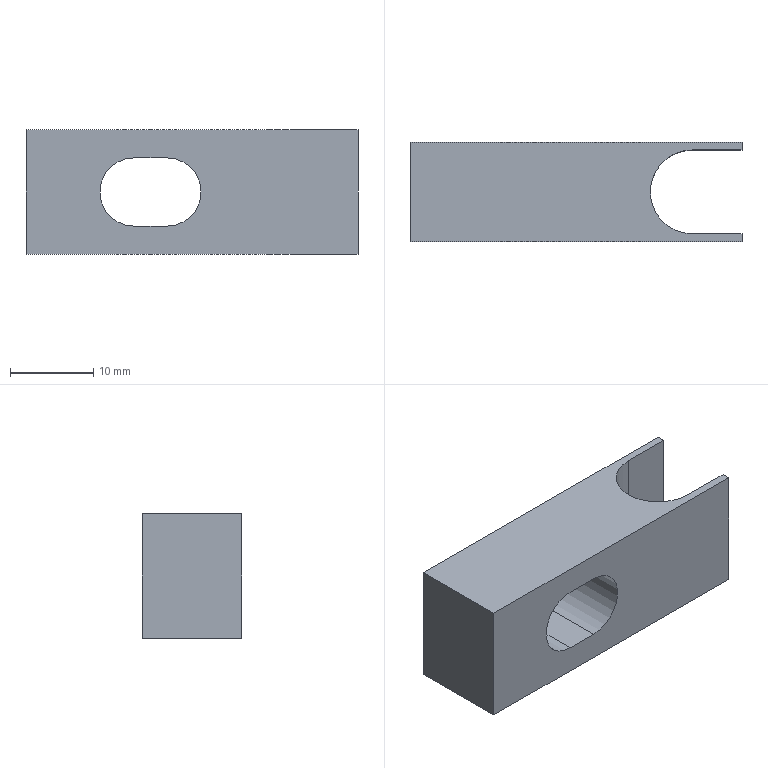Part | STEP file | Lead screw movable block QY-1-18 | 1 solid | 15 faces | box 40 x 12 x 15 mm | volume 4663 mm3 | plane 11 | cylinder 4 | commonest cylinder face diameters 8.2 x2 10.1 x2
STEP:
#1=CARTESIAN_POINT('',(0.,0.,0.));
#2=DIRECTION('',(0.,0.,1.));
#3=DIRECTION('',(1.,0.,0.));
#4=AXIS2_PLACEMENT_3D('',#1,#2,#3);
#5=CARTESIAN_POINT('',(9.9,2.027,15.));
#6=VERTEX_POINT('',#5);
#7=CARTESIAN_POINT('',(9.9,2.027,0.));
#8=VERTEX_POINT('',#7);
#9=CARTESIAN_POINT('',(9.9,2.027,15.));
#10=DIRECTION('',(0.,0.,-1.));
#11=VECTOR('',#10,1.);
#12=LINE('',#9,#11);
#13=CARTESIAN_POINT('',(9.9,-3.023,15.));
#14=DIRECTION('',(0.,0.,-1.));
#15=DIRECTION('',(-1.,0.,0.));
#16=AXIS2_PLACEMENT_3D('',#13,#14,#15);
#17=CYLINDRICAL_SURFACE('',#16,5.05);
#18=CARTESIAN_POINT('',(1.571,0.));
#19=DIRECTION('',(0.,1.));
#20=VECTOR('',#19,1.);
#21=LINE('',#18,#20);
#22=(GEOMETRIC_REPRESENTATION_CONTEXT(2)PARAMETRIC_REPRESENTATION_CONTEXT()REPRESENTATION_CONTEXT('',''));
#23=DEFINITIONAL_REPRESENTATION('',(#21),#22);
#24=PCURVE('',#17,#23);
#25=CARTESIAN_POINT('',(9.9,2.027,15.));
#26=DIRECTION('',(0.,1.,0.));
#27=DIRECTION('',(0.,0.,1.));
#28=AXIS2_PLACEMENT_3D('',#25,#26,#27);
#29=PLANE('',#28);
#30=CARTESIAN_POINT('',(0.,0.));
#31=DIRECTION('',(-1.,0.));
#32=VECTOR('',#31,1.);
#33=LINE('',#30,#32);
#34=(GEOMETRIC_REPRESENTATION_CONTEXT(2)PARAMETRIC_REPRESENTATION_CONTEXT()REPRESENTATION_CONTEXT('',''));
#35=DEFINITIONAL_REPRESENTATION('',(#33),#34);
#36=PCURVE('',#29,#35);
#37=SURFACE_CURVE('',#12,(#24,#36),.PCURVE_S1.);
#38=EDGE_CURVE('',#6,#8,#37,.T.);
#39=ORIENTED_EDGE('',*,*,#38,.T.);
#40=CARTESIAN_POINT('',(4.85,-3.023,0.));
#41=VERTEX_POINT('',#40);
#42=CARTESIAN_POINT('',(9.9,-3.023,0.));
#43=DIRECTION('',(0.,0.,-1.));
#44=DIRECTION('',(1.,0.,0.));
#45=AXIS2_PLACEMENT_3D('',#42,#43,#44);
#46=CIRCLE('',#45,5.05);
#47=CARTESIAN_POINT('',(-3.142,15.));
#48=DIRECTION('',(1.,0.));
#49=VECTOR('',#48,1.);
#50=LINE('',#47,#49);
#51=(GEOMETRIC_REPRESENTATION_CONTEXT(2)PARAMETRIC_REPRESENTATION_CONTEXT()REPRESENTATION_CONTEXT('',''));
#52=DEFINITIONAL_REPRESENTATION('',(#50),#51);
#53=PCURVE('',#17,#52);
#54=CARTESIAN_POINT('',(9.9,-3.023,0.));
#55=DIRECTION('',(0.,0.,1.));
#56=DIRECTION('',(1.,0.,0.));
#57=AXIS2_PLACEMENT_3D('',#54,#55,#56);
#58=PLANE('',#57);
#59=CARTESIAN_POINT('',(5.05,0.));
#60=CARTESIAN_POINT('',(5.05,-8.747));
#61=CARTESIAN_POINT('',(-2.525,-4.373));
#62=CARTESIAN_POINT('',(-10.1,0.));
#63=CARTESIAN_POINT('',(-2.525,4.373));
#64=CARTESIAN_POINT('',(5.05,8.747));
#65=CARTESIAN_POINT('',(5.05,0.));
#66=(BOUNDED_CURVE()B_SPLINE_CURVE(2,(#59,#60,#61,#62,#63,#64,#65),.UNSPECIFIED.,.T.,.F.)B_SPLINE_CURVE_WITH_KNOTS((1,2,2,2,2,1),(-2.094,0.,2.094,4.189,6.283,8.378),.UNSPECIFIED.)CURVE()GEOMETRIC_REPRESENTATION_ITEM()RATIONAL_B_SPLINE_CURVE((1.,0.5,1.,0.5,1.,0.5,1.))REPRESENTATION_ITEM(''));
#67=(GEOMETRIC_REPRESENTATION_CONTEXT(2)PARAMETRIC_REPRESENTATION_CONTEXT()REPRESENTATION_CONTEXT('',''));
#68=DEFINITIONAL_REPRESENTATION('',(#66),#67);
#69=PCURVE('',#58,#68);
#70=SURFACE_CURVE('',#46,(#53,#69),.PCURVE_S1.);
#71=EDGE_CURVE('',#41,#8,#70,.T.);
#72=ORIENTED_EDGE('',*,*,#71,.F.);
#73=CARTESIAN_POINT('',(4.85,-3.023,15.));
#74=VERTEX_POINT('',#73);
#75=CARTESIAN_POINT('',(4.85,-3.023,15.));
#76=DIRECTION('',(0.,0.,-1.));
#77=VECTOR('',#76,1.);
#78=LINE('',#75,#77);
#79=CARTESIAN_POINT('',(0.,0.));
#80=DIRECTION('',(0.,1.));
#81=VECTOR('',#80,1.);
#82=LINE('',#79,#81);
#83=(GEOMETRIC_REPRESENTATION_CONTEXT(2)PARAMETRIC_REPRESENTATION_CONTEXT()REPRESENTATION_CONTEXT('',''));
#84=DEFINITIONAL_REPRESENTATION('',(#82),#83);
#85=PCURVE('',#17,#84);
#86=CARTESIAN_POINT('',(9.9,-3.023,15.));
#87=DIRECTION('',(0.,0.,-1.));
#88=DIRECTION('',(-1.,0.,0.));
#89=AXIS2_PLACEMENT_3D('',#86,#87,#88);
#90=CYLINDRICAL_SURFACE('',#89,5.05);
#91=CARTESIAN_POINT('',(6.283,0.));
#92=DIRECTION('',(0.,1.));
#93=VECTOR('',#92,1.);
#94=LINE('',#91,#93);
#95=(GEOMETRIC_REPRESENTATION_CONTEXT(2)PARAMETRIC_REPRESENTATION_CONTEXT()REPRESENTATION_CONTEXT('',''));
#96=DEFINITIONAL_REPRESENTATION('',(#94),#95);
#97=PCURVE('',#90,#96);
#98=SURFACE_CURVE('',#78,(#85,#97),.PCURVE_S1.);
#99=EDGE_CURVE('',#74,#41,#98,.T.);
#100=ORIENTED_EDGE('',*,*,#99,.F.);
#101=CARTESIAN_POINT('',(9.9,-3.023,15.));
#102=DIRECTION('',(0.,0.,-1.));
#103=DIRECTION('',(1.,0.,0.));
#104=AXIS2_PLACEMENT_3D('',#101,#102,#103);
#105=CIRCLE('',#104,5.05);
#106=CARTESIAN_POINT('',(-3.142,0.));
#107=DIRECTION('',(1.,0.));
#108=VECTOR('',#107,1.);
#109=LINE('',#106,#108);
#110=(GEOMETRIC_REPRESENTATION_CONTEXT(2)PARAMETRIC_REPRESENTATION_CONTEXT()REPRESENTATION_CONTEXT('',''));
#111=DEFINITIONAL_REPRESENTATION('',(#109),#110);
#112=PCURVE('',#17,#111);
#113=CARTESIAN_POINT('',(9.9,-3.023,15.));
#114=DIRECTION('',(0.,0.,1.));
#115=DIRECTION('',(1.,0.,0.));
#116=AXIS2_PLACEMENT_3D('',#113,#114,#115);
#117=PLANE('',#116);
#118=CARTESIAN_POINT('',(5.05,0.));
#119=CARTESIAN_POINT('',(5.05,-8.747));
#120=CARTESIAN_POINT('',(-2.525,-4.373));
#121=CARTESIAN_POINT('',(-10.1,0.));
#122=CARTESIAN_POINT('',(-2.525,4.373));
#123=CARTESIAN_POINT('',(5.05,8.747));
#124=CARTESIAN_POINT('',(5.05,0.));
#125=(BOUNDED_CURVE()B_SPLINE_CURVE(2,(#118,#119,#120,#121,#122,#123,#124),.UNSPECIFIED.,.T.,.F.)B_SPLINE_CURVE_WITH_KNOTS((1,2,2,2,2,1),(-2.094,0.,2.094,4.189,6.283,8.378),.UNSPECIFIED.)CURVE()GEOMETRIC_REPRESENTATION_ITEM()RATIONAL_B_SPLINE_CURVE((1.,0.5,1.,0.5,1.,0.5,1.))REPRESENTATION_ITEM(''));
#126=(GEOMETRIC_REPRESENTATION_CONTEXT(2)PARAMETRIC_REPRESENTATION_CONTEXT()REPRESENTATION_CONTEXT('',''));
#127=DEFINITIONAL_REPRESENTATION('',(#125),#126);
#128=PCURVE('',#117,#127);
#129=SURFACE_CURVE('',#105,(#112,#128),.PCURVE_S1.);
#130=EDGE_CURVE('',#74,#6,#129,.T.);
#131=ORIENTED_EDGE('',*,*,#130,.T.);
#132=EDGE_LOOP('',(#39,#72,#100,#131));
#133=FACE_BOUND('',#132,.F.);
#134=ADVANCED_FACE('',(#133),#17,.F.);
#135=CARTESIAN_POINT('',(-24.1,2.977,0.));
#136=VERTEX_POINT('',#135);
#137=CARTESIAN_POINT('',(-24.1,-9.023,0.));
#138=VERTEX_POINT('',#137);
#139=CARTESIAN_POINT('',(-24.1,2.977,0.));
#140=DIRECTION('',(0.,-1.,0.));
#141=VECTOR('',#140,1.);
#142=LINE('',#139,#141);
#143=CARTESIAN_POINT('',(-24.1,2.977,15.));
#144=DIRECTION('',(1.,0.,0.));
#145=DIRECTION('',(0.,0.,-1.));
#146=AXIS2_PLACEMENT_3D('',#143,#144,#145);
#147=PLANE('',#146);
#148=CARTESIAN_POINT('',(15.,0.));
#149=DIRECTION('',(0.,-1.));
#150=VECTOR('',#149,1.);
#151=LINE('',#148,#150);
#152=(GEOMETRIC_REPRESENTATION_CONTEXT(2)PARAMETRIC_REPRESENTATION_CONTEXT()REPRESENTATION_CONTEXT('',''));
#153=DEFINITIONAL_REPRESENTATION('',(#151),#152);
#154=PCURVE('',#147,#153);
#155=CARTESIAN_POINT('',(-34.,6.));
#156=DIRECTION('',(0.,-1.));
#157=VECTOR('',#156,1.);
#158=LINE('',#155,#157);
#159=(GEOMETRIC_REPRESENTATION_CONTEXT(2)PARAMETRIC_REPRESENTATION_CONTEXT()REPRESENTATION_CONTEXT('',''));
#160=DEFINITIONAL_REPRESENTATION('',(#158),#159);
#161=PCURVE('',#58,#160);
#162=SURFACE_CURVE('',#142,(#154,#161),.PCURVE_S1.);
#163=EDGE_CURVE('',#136,#138,#162,.T.);
#164=ORIENTED_EDGE('',*,*,#163,.T.);
#165=CARTESIAN_POINT('',(-24.1,-9.023,15.));
#166=VERTEX_POINT('',#165);
#167=CARTESIAN_POINT('',(-24.1,-9.023,15.));
#168=DIRECTION('',(0.,0.,-1.));
#169=VECTOR('',#168,1.);
#170=LINE('',#167,#169);
#171=CARTESIAN_POINT('',(0.,-12.));
#172=DIRECTION('',(1.,0.));
#173=VECTOR('',#172,1.);
#174=LINE('',#171,#173);
#175=(GEOMETRIC_REPRESENTATION_CONTEXT(2)PARAMETRIC_REPRESENTATION_CONTEXT()REPRESENTATION_CONTEXT('',''));
#176=DEFINITIONAL_REPRESENTATION('',(#174),#175);
#177=PCURVE('',#147,#176);
#178=CARTESIAN_POINT('',(-24.1,-9.023,15.));
#179=DIRECTION('',(0.,1.,0.));
#180=DIRECTION('',(0.,0.,1.));
#181=AXIS2_PLACEMENT_3D('',#178,#179,#180);
#182=PLANE('',#181);
#183=CARTESIAN_POINT('',(0.,0.));
#184=DIRECTION('',(-1.,0.));
#185=VECTOR('',#184,1.);
#186=LINE('',#183,#185);
#187=(GEOMETRIC_REPRESENTATION_CONTEXT(2)PARAMETRIC_REPRESENTATION_CONTEXT()REPRESENTATION_CONTEXT('',''));
#188=DEFINITIONAL_REPRESENTATION('',(#186),#187);
#189=PCURVE('',#182,#188);
#190=SURFACE_CURVE('',#170,(#177,#189),.PCURVE_S1.);
#191=EDGE_CURVE('',#166,#138,#190,.T.);
#192=ORIENTED_EDGE('',*,*,#191,.F.);
#193=CARTESIAN_POINT('',(-24.1,2.977,15.));
#194=VERTEX_POINT('',#193);
#195=CARTESIAN_POINT('',(-24.1,2.977,15.));
#196=DIRECTION('',(0.,-1.,0.));
#197=VECTOR('',#196,1.);
#198=LINE('',#195,#197);
#199=CARTESIAN_POINT('',(0.,0.));
#200=DIRECTION('',(0.,-1.));
#201=VECTOR('',#200,1.);
#202=LINE('',#199,#201);
#203=(GEOMETRIC_REPRESENTATION_CONTEXT(2)PARAMETRIC_REPRESENTATION_CONTEXT()REPRESENTATION_CONTEXT('',''));
#204=DEFINITIONAL_REPRESENTATION('',(#202),#203);
#205=PCURVE('',#147,#204);
#206=CARTESIAN_POINT('',(-34.,6.));
#207=DIRECTION('',(0.,-1.));
#208=VECTOR('',#207,1.);
#209=LINE('',#206,#208);
#210=(GEOMETRIC_REPRESENTATION_CONTEXT(2)PARAMETRIC_REPRESENTATION_CONTEXT()REPRESENTATION_CONTEXT('',''));
#211=DEFINITIONAL_REPRESENTATION('',(#209),#210);
#212=PCURVE('',#117,#211);
#213=SURFACE_CURVE('',#198,(#205,#212),.PCURVE_S1.);
#214=EDGE_CURVE('',#194,#166,#213,.T.);
#215=ORIENTED_EDGE('',*,*,#214,.F.);
#216=CARTESIAN_POINT('',(-24.1,2.977,15.));
#217=DIRECTION('',(0.,0.,-1.));
#218=VECTOR('',#217,1.);
#219=LINE('',#216,#218);
#220=CARTESIAN_POINT('',(0.,0.));
#221=DIRECTION('',(1.,0.));
#222=VECTOR('',#221,1.);
#223=LINE('',#220,#222);
#224=(GEOMETRIC_REPRESENTATION_CONTEXT(2)PARAMETRIC_REPRESENTATION_CONTEXT()REPRESENTATION_CONTEXT('',''));
#225=DEFINITIONAL_REPRESENTATION('',(#223),#224);
#226=PCURVE('',#147,#225);
#227=CARTESIAN_POINT('',(-24.1,2.977,15.));
#228=DIRECTION('',(0.,-1.,0.));
#229=DIRECTION('',(1.,0.,0.));
#230=AXIS2_PLACEMENT_3D('',#227,#228,#229);
#231=PLANE('',#230);
#232=CARTESIAN_POINT('',(0.,0.));
#233=DIRECTION('',(0.,-1.));
#234=VECTOR('',#233,1.);
#235=LINE('',#232,#234);
#236=(GEOMETRIC_REPRESENTATION_CONTEXT(2)PARAMETRIC_REPRESENTATION_CONTEXT()REPRESENTATION_CONTEXT('',''));
#237=DEFINITIONAL_REPRESENTATION('',(#235),#236);
#238=PCURVE('',#231,#237);
#239=SURFACE_CURVE('',#219,(#226,#238),.PCURVE_S1.);
#240=EDGE_CURVE('',#194,#136,#239,.T.);
#241=ORIENTED_EDGE('',*,*,#240,.T.);
#242=EDGE_LOOP('',(#164,#192,#215,#241));
#243=FACE_BOUND('',#242,.T.);
#244=ADVANCED_FACE('',(#243),#147,.F.);
#245=CARTESIAN_POINT('',(-7.1,-9.023,11.6));
#246=VERTEX_POINT('',#245);
#247=CARTESIAN_POINT('',(-11.1,-9.023,11.6));
#248=VERTEX_POINT('',#247);
#249=CARTESIAN_POINT('',(-7.1,-9.023,11.6));
#250=DIRECTION('',(-1.,0.,0.));
#251=VECTOR('',#250,1.);
#252=LINE('',#249,#251);
#253=CARTESIAN_POINT('',(-3.4,17.));
#254=DIRECTION('',(0.,-1.));
#255=VECTOR('',#254,1.);
#256=LINE('',#253,#255);
#257=(GEOMETRIC_REPRESENTATION_CONTEXT(2)PARAMETRIC_REPRESENTATION_CONTEXT()REPRESENTATION_CONTEXT('',''));
#258=DEFINITIONAL_REPRESENTATION('',(#256),#257);
#259=PCURVE('',#182,#258);
#260=CARTESIAN_POINT('',(-7.1,5.977,11.6));
#261=DIRECTION('',(0.,0.,1.));
#262=DIRECTION('',(1.,0.,0.));
#263=AXIS2_PLACEMENT_3D('',#260,#261,#262);
#264=PLANE('',#263);
#265=CARTESIAN_POINT('',(0.,-15.));
#266=DIRECTION('',(-1.,0.));
#267=VECTOR('',#266,1.);
#268=LINE('',#265,#267);
#269=(GEOMETRIC_REPRESENTATION_CONTEXT(2)PARAMETRIC_REPRESENTATION_CONTEXT()REPRESENTATION_CONTEXT('',''));
#270=DEFINITIONAL_REPRESENTATION('',(#268),#269);
#271=PCURVE('',#264,#270);
#272=SURFACE_CURVE('',#252,(#259,#271),.PCURVE_S1.);
#273=EDGE_CURVE('',#246,#248,#272,.T.);
#274=ORIENTED_EDGE('',*,*,#273,.F.);
#275=CARTESIAN_POINT('',(-7.1,-9.023,3.4));
#276=VERTEX_POINT('',#275);
#277=CARTESIAN_POINT('',(-7.1,-9.023,7.5));
#278=DIRECTION('',(0.,-1.,0.));
#279=DIRECTION('',(0.,0.,-1.));
#280=AXIS2_PLACEMENT_3D('',#277,#278,#279);
#281=CIRCLE('',#280,4.1);
#282=CARTESIAN_POINT('',(-11.6,17.));
#283=CARTESIAN_POINT('',(-11.6,24.101));
#284=CARTESIAN_POINT('',(-5.45,20.551));
#285=CARTESIAN_POINT('',(0.7,17.));
#286=CARTESIAN_POINT('',(-5.45,13.449));
#287=CARTESIAN_POINT('',(-11.6,9.899));
#288=CARTESIAN_POINT('',(-11.6,17.));
#289=(BOUNDED_CURVE()B_SPLINE_CURVE(2,(#282,#283,#284,#285,#286,#287,#288),.UNSPECIFIED.,.T.,.F.)B_SPLINE_CURVE_WITH_KNOTS((1,2,2,2,2,1),(-2.094,0.,2.094,4.189,6.283,8.378),.UNSPECIFIED.)CURVE()GEOMETRIC_REPRESENTATION_ITEM()RATIONAL_B_SPLINE_CURVE((1.,0.5,1.,0.5,1.,0.5,1.))REPRESENTATION_ITEM(''));
#290=(GEOMETRIC_REPRESENTATION_CONTEXT(2)PARAMETRIC_REPRESENTATION_CONTEXT()REPRESENTATION_CONTEXT('',''));
#291=DEFINITIONAL_REPRESENTATION('',(#289),#290);
#292=PCURVE('',#182,#291);
#293=CARTESIAN_POINT('',(-7.1,5.977,7.5));
#294=DIRECTION('',(0.,-1.,0.));
#295=DIRECTION('',(0.,0.,-1.));
#296=AXIS2_PLACEMENT_3D('',#293,#294,#295);
#297=CYLINDRICAL_SURFACE('',#296,4.1);
#298=CARTESIAN_POINT('',(0.,15.));
#299=DIRECTION('',(1.,0.));
#300=VECTOR('',#299,1.);
#301=LINE('',#298,#300);
#302=(GEOMETRIC_REPRESENTATION_CONTEXT(2)PARAMETRIC_REPRESENTATION_CONTEXT()REPRESENTATION_CONTEXT('',''));
#303=DEFINITIONAL_REPRESENTATION('',(#301),#302);
#304=PCURVE('',#297,#303);
#305=SURFACE_CURVE('',#281,(#292,#304),.PCURVE_S1.);
#306=EDGE_CURVE('',#276,#246,#305,.T.);
#307=ORIENTED_EDGE('',*,*,#306,.F.);
#308=CARTESIAN_POINT('',(-11.1,-9.023,3.4));
#309=VERTEX_POINT('',#308);
#310=CARTESIAN_POINT('',(-7.1,-9.023,3.4));
#311=DIRECTION('',(1.,0.,0.));
#312=VECTOR('',#311,1.);
#313=LINE('',#310,#312);
#314=CARTESIAN_POINT('',(-11.6,17.));
#315=DIRECTION('',(0.,1.));
#316=VECTOR('',#315,1.);
#317=LINE('',#314,#316);
#318=(GEOMETRIC_REPRESENTATION_CONTEXT(2)PARAMETRIC_REPRESENTATION_CONTEXT()REPRESENTATION_CONTEXT('',''));
#319=DEFINITIONAL_REPRESENTATION('',(#317),#318);
#320=PCURVE('',#182,#319);
#321=CARTESIAN_POINT('',(-7.1,5.977,3.4));
#322=DIRECTION('',(0.,0.,-1.));
#323=DIRECTION('',(-1.,0.,0.));
#324=AXIS2_PLACEMENT_3D('',#321,#322,#323);
#325=PLANE('',#324);
#326=CARTESIAN_POINT('',(0.,-15.));
#327=DIRECTION('',(-1.,0.));
#328=VECTOR('',#327,1.);
#329=LINE('',#326,#328);
#330=(GEOMETRIC_REPRESENTATION_CONTEXT(2)PARAMETRIC_REPRESENTATION_CONTEXT()REPRESENTATION_CONTEXT('',''));
#331=DEFINITIONAL_REPRESENTATION('',(#329),#330);
#332=PCURVE('',#325,#331);
#333=SURFACE_CURVE('',#313,(#320,#332),.PCURVE_S1.);
#334=EDGE_CURVE('',#309,#276,#333,.T.);
#335=ORIENTED_EDGE('',*,*,#334,.F.);
#336=CARTESIAN_POINT('',(-11.1,-9.023,7.5));
#337=DIRECTION('',(0.,-1.,0.));
#338=DIRECTION('',(0.,0.,-1.));
#339=AXIS2_PLACEMENT_3D('',#336,#337,#338);
#340=CIRCLE('',#339,4.1);
#341=CARTESIAN_POINT('',(-11.6,13.));
#342=CARTESIAN_POINT('',(-11.6,20.101));
#343=CARTESIAN_POINT('',(-5.45,16.551));
#344=CARTESIAN_POINT('',(0.7,13.));
#345=CARTESIAN_POINT('',(-5.45,9.449));
#346=CARTESIAN_POINT('',(-11.6,5.899));
#347=CARTESIAN_POINT('',(-11.6,13.));
#348=(BOUNDED_CURVE()B_SPLINE_CURVE(2,(#341,#342,#343,#344,#345,#346,#347),.UNSPECIFIED.,.T.,.F.)B_SPLINE_CURVE_WITH_KNOTS((1,2,2,2,2,1),(-2.094,0.,2.094,4.189,6.283,8.378),.UNSPECIFIED.)CURVE()GEOMETRIC_REPRESENTATION_ITEM()RATIONAL_B_SPLINE_CURVE((1.,0.5,1.,0.5,1.,0.5,1.))REPRESENTATION_ITEM(''));
#349=(GEOMETRIC_REPRESENTATION_CONTEXT(2)PARAMETRIC_REPRESENTATION_CONTEXT()REPRESENTATION_CONTEXT('',''));
#350=DEFINITIONAL_REPRESENTATION('',(#348),#349);
#351=PCURVE('',#182,#350);
#352=CARTESIAN_POINT('',(-11.1,5.977,7.5));
#353=DIRECTION('',(0.,-1.,0.));
#354=DIRECTION('',(0.,0.,-1.));
#355=AXIS2_PLACEMENT_3D('',#352,#353,#354);
#356=CYLINDRICAL_SURFACE('',#355,4.1);
#357=CARTESIAN_POINT('',(0.,15.));
#358=DIRECTION('',(1.,0.));
#359=VECTOR('',#358,1.);
#360=LINE('',#357,#359);
#361=(GEOMETRIC_REPRESENTATION_CONTEXT(2)PARAMETRIC_REPRESENTATION_CONTEXT()REPRESENTATION_CONTEXT('',''));
#362=DEFINITIONAL_REPRESENTATION('',(#360),#361);
#363=PCURVE('',#356,#362);
#364=SURFACE_CURVE('',#340,(#351,#363),.PCURVE_S1.);
#365=EDGE_CURVE('',#248,#309,#364,.T.);
#366=ORIENTED_EDGE('',*,*,#365,.F.);
#367=EDGE_LOOP('',(#274,#307,#335,#366));
#368=FACE_BOUND('',#367,.T.);
#369=CARTESIAN_POINT('',(15.9,-9.023,0.));
#370=VERTEX_POINT('',#369);
#371=CARTESIAN_POINT('',(-24.1,-9.023,0.));
#372=DIRECTION('',(1.,0.,0.));
#373=VECTOR('',#372,1.);
#374=LINE('',#371,#373);
#375=CARTESIAN_POINT('',(-15.,0.));
#376=DIRECTION('',(0.,1.));
#377=VECTOR('',#376,1.);
#378=LINE('',#375,#377);
#379=(GEOMETRIC_REPRESENTATION_CONTEXT(2)PARAMETRIC_REPRESENTATION_CONTEXT()REPRESENTATION_CONTEXT('',''));
#380=DEFINITIONAL_REPRESENTATION('',(#378),#379);
#381=PCURVE('',#182,#380);
#382=CARTESIAN_POINT('',(-34.,-6.));
#383=DIRECTION('',(1.,0.));
#384=VECTOR('',#383,1.);
#385=LINE('',#382,#384);
#386=(GEOMETRIC_REPRESENTATION_CONTEXT(2)PARAMETRIC_REPRESENTATION_CONTEXT()REPRESENTATION_CONTEXT('',''));
#387=DEFINITIONAL_REPRESENTATION('',(#385),#386);
#388=PCURVE('',#58,#387);
#389=SURFACE_CURVE('',#374,(#381,#388),.PCURVE_S1.);
#390=EDGE_CURVE('',#138,#370,#389,.T.);
#391=ORIENTED_EDGE('',*,*,#390,.T.);
#392=CARTESIAN_POINT('',(15.9,-9.023,15.));
#393=VERTEX_POINT('',#392);
#394=CARTESIAN_POINT('',(15.9,-9.023,15.));
#395=DIRECTION('',(0.,0.,-1.));
#396=VECTOR('',#395,1.);
#397=LINE('',#394,#396);
#398=CARTESIAN_POINT('',(0.,40.));
#399=DIRECTION('',(-1.,0.));
#400=VECTOR('',#399,1.);
#401=LINE('',#398,#400);
#402=(GEOMETRIC_REPRESENTATION_CONTEXT(2)PARAMETRIC_REPRESENTATION_CONTEXT()REPRESENTATION_CONTEXT('',''));
#403=DEFINITIONAL_REPRESENTATION('',(#401),#402);
#404=PCURVE('',#182,#403);
#405=CARTESIAN_POINT('',(15.9,-8.073,15.));
#406=DIRECTION('',(-1.,0.,0.));
#407=DIRECTION('',(0.,0.,1.));
#408=AXIS2_PLACEMENT_3D('',#405,#406,#407);
#409=PLANE('',#408);
#410=CARTESIAN_POINT('',(0.,-0.95));
#411=DIRECTION('',(-1.,0.));
#412=VECTOR('',#411,1.);
#413=LINE('',#410,#412);
#414=(GEOMETRIC_REPRESENTATION_CONTEXT(2)PARAMETRIC_REPRESENTATION_CONTEXT()REPRESENTATION_CONTEXT('',''));
#415=DEFINITIONAL_REPRESENTATION('',(#413),#414);
#416=PCURVE('',#409,#415);
#417=SURFACE_CURVE('',#397,(#404,#416),.PCURVE_S1.);
#418=EDGE_CURVE('',#393,#370,#417,.T.);
#419=ORIENTED_EDGE('',*,*,#418,.F.);
#420=CARTESIAN_POINT('',(-24.1,-9.023,15.));
#421=DIRECTION('',(1.,0.,0.));
#422=VECTOR('',#421,1.);
#423=LINE('',#420,#422);
#424=CARTESIAN_POINT('',(0.,0.));
#425=DIRECTION('',(0.,1.));
#426=VECTOR('',#425,1.);
#427=LINE('',#424,#426);
#428=(GEOMETRIC_REPRESENTATION_CONTEXT(2)PARAMETRIC_REPRESENTATION_CONTEXT()REPRESENTATION_CONTEXT('',''));
#429=DEFINITIONAL_REPRESENTATION('',(#427),#428);
#430=PCURVE('',#182,#429);
#431=CARTESIAN_POINT('',(-34.,-6.));
#432=DIRECTION('',(1.,0.));
#433=VECTOR('',#432,1.);
#434=LINE('',#431,#433);
#435=(GEOMETRIC_REPRESENTATION_CONTEXT(2)PARAMETRIC_REPRESENTATION_CONTEXT()REPRESENTATION_CONTEXT('',''));
#436=DEFINITIONAL_REPRESENTATION('',(#434),#435);
#437=PCURVE('',#117,#436);
#438=SURFACE_CURVE('',#423,(#430,#437),.PCURVE_S1.);
#439=EDGE_CURVE('',#166,#393,#438,.T.);
#440=ORIENTED_EDGE('',*,*,#439,.F.);
#441=ORIENTED_EDGE('',*,*,#191,.T.);
#442=EDGE_LOOP('',(#391,#419,#440,#441));
#443=FACE_BOUND('',#442,.T.);
#444=ADVANCED_FACE('',(#368,#443),#182,.F.);
#445=CARTESIAN_POINT('',(15.9,-8.073,0.));
#446=VERTEX_POINT('',#445);
#447=CARTESIAN_POINT('',(15.9,-8.073,0.));
#448=DIRECTION('',(0.,1.,0.));
#449=VECTOR('',#448,1.);
#450=LINE('',#447,#449);
#451=CARTESIAN_POINT('',(-15.,0.));
#452=DIRECTION('',(0.,1.));
#453=VECTOR('',#452,1.);
#454=LINE('',#451,#453);
#455=(GEOMETRIC_REPRESENTATION_CONTEXT(2)PARAMETRIC_REPRESENTATION_CONTEXT()REPRESENTATION_CONTEXT('',''));
#456=DEFINITIONAL_REPRESENTATION('',(#454),#455);
#457=PCURVE('',#409,#456);
#458=CARTESIAN_POINT('',(6.,-5.05));
#459=DIRECTION('',(0.,1.));
#460=VECTOR('',#459,1.);
#461=LINE('',#458,#460);
#462=(GEOMETRIC_REPRESENTATION_CONTEXT(2)PARAMETRIC_REPRESENTATION_CONTEXT()REPRESENTATION_CONTEXT('',''));
#463=DEFINITIONAL_REPRESENTATION('',(#461),#462);
#464=PCURVE('',#58,#463);
#465=SURFACE_CURVE('',#450,(#457,#464),.PCURVE_S1.);
#466=EDGE_CURVE('',#370,#446,#465,.T.);
#467=ORIENTED_EDGE('',*,*,#466,.T.);
#468=CARTESIAN_POINT('',(15.9,-8.073,15.));
#469=VERTEX_POINT('',#468);
#470=CARTESIAN_POINT('',(15.9,-8.073,15.));
#471=DIRECTION('',(0.,0.,-1.));
#472=VECTOR('',#471,1.);
#473=LINE('',#470,#472);
#474=CARTESIAN_POINT('',(0.,0.));
#475=DIRECTION('',(-1.,0.));
#476=VECTOR('',#475,1.);
#477=LINE('',#474,#476);
#478=(GEOMETRIC_REPRESENTATION_CONTEXT(2)PARAMETRIC_REPRESENTATION_CONTEXT()REPRESENTATION_CONTEXT('',''));
#479=DEFINITIONAL_REPRESENTATION('',(#477),#478);
#480=PCURVE('',#409,#479);
#481=CARTESIAN_POINT('',(9.9,-8.073,15.));
#482=DIRECTION('',(0.,-1.,0.));
#483=DIRECTION('',(0.,0.,-1.));
#484=AXIS2_PLACEMENT_3D('',#481,#482,#483);
#485=PLANE('',#484);
#486=CARTESIAN_POINT('',(0.,6.));
#487=DIRECTION('',(1.,0.));
#488=VECTOR('',#487,1.);
#489=LINE('',#486,#488);
#490=(GEOMETRIC_REPRESENTATION_CONTEXT(2)PARAMETRIC_REPRESENTATION_CONTEXT()REPRESENTATION_CONTEXT('',''));
#491=DEFINITIONAL_REPRESENTATION('',(#489),#490);
#492=PCURVE('',#485,#491);
#493=SURFACE_CURVE('',#473,(#480,#492),.PCURVE_S1.);
#494=EDGE_CURVE('',#469,#446,#493,.T.);
#495=ORIENTED_EDGE('',*,*,#494,.F.);
#496=CARTESIAN_POINT('',(15.9,-8.073,15.));
#497=DIRECTION('',(0.,1.,0.));
#498=VECTOR('',#497,1.);
#499=LINE('',#496,#498);
#500=CARTESIAN_POINT('',(0.,0.));
#501=DIRECTION('',(0.,1.));
#502=VECTOR('',#501,1.);
#503=LINE('',#500,#502);
#504=(GEOMETRIC_REPRESENTATION_CONTEXT(2)PARAMETRIC_REPRESENTATION_CONTEXT()REPRESENTATION_CONTEXT('',''));
#505=DEFINITIONAL_REPRESENTATION('',(#503),#504);
#506=PCURVE('',#409,#505);
#507=CARTESIAN_POINT('',(6.,-5.05));
#508=DIRECTION('',(0.,1.));
#509=VECTOR('',#508,1.);
#510=LINE('',#507,#509);
#511=(GEOMETRIC_REPRESENTATION_CONTEXT(2)PARAMETRIC_REPRESENTATION_CONTEXT()REPRESENTATION_CONTEXT('',''));
#512=DEFINITIONAL_REPRESENTATION('',(#510),#511);
#513=PCURVE('',#117,#512);
#514=SURFACE_CURVE('',#499,(#506,#513),.PCURVE_S1.);
#515=EDGE_CURVE('',#393,#469,#514,.T.);
#516=ORIENTED_EDGE('',*,*,#515,.F.);
#517=ORIENTED_EDGE('',*,*,#418,.T.);
#518=EDGE_LOOP('',(#467,#495,#516,#517));
#519=FACE_BOUND('',#518,.T.);
#520=ADVANCED_FACE('',(#519),#409,.F.);
#521=CARTESIAN_POINT('',(9.9,-8.073,0.));
#522=VERTEX_POINT('',#521);
#523=CARTESIAN_POINT('',(9.9,-8.073,0.));
#524=DIRECTION('',(-1.,0.,0.));
#525=VECTOR('',#524,1.);
#526=LINE('',#523,#525);
#527=CARTESIAN_POINT('',(15.,0.));
#528=DIRECTION('',(0.,-1.));
#529=VECTOR('',#528,1.);
#530=LINE('',#527,#529);
#531=(GEOMETRIC_REPRESENTATION_CONTEXT(2)PARAMETRIC_REPRESENTATION_CONTEXT()REPRESENTATION_CONTEXT('',''));
#532=DEFINITIONAL_REPRESENTATION('',(#530),#531);
#533=PCURVE('',#485,#532);
#534=CARTESIAN_POINT('',(0.,-5.05));
#535=DIRECTION('',(-1.,0.));
#536=VECTOR('',#535,1.);
#537=LINE('',#534,#536);
#538=(GEOMETRIC_REPRESENTATION_CONTEXT(2)PARAMETRIC_REPRESENTATION_CONTEXT()REPRESENTATION_CONTEXT('',''));
#539=DEFINITIONAL_REPRESENTATION('',(#537),#538);
#540=PCURVE('',#58,#539);
#541=SURFACE_CURVE('',#526,(#533,#540),.PCURVE_S1.);
#542=EDGE_CURVE('',#446,#522,#541,.T.);
#543=ORIENTED_EDGE('',*,*,#542,.T.);
#544=CARTESIAN_POINT('',(9.9,-8.073,15.));
#545=VERTEX_POINT('',#544);
#546=CARTESIAN_POINT('',(9.9,-8.073,15.));
#547=DIRECTION('',(0.,0.,-1.));
#548=VECTOR('',#547,1.);
#549=LINE('',#546,#548);
#550=CARTESIAN_POINT('',(0.,0.));
#551=DIRECTION('',(1.,0.));
#552=VECTOR('',#551,1.);
#553=LINE('',#550,#552);
#554=(GEOMETRIC_REPRESENTATION_CONTEXT(2)PARAMETRIC_REPRESENTATION_CONTEXT()REPRESENTATION_CONTEXT('',''));
#555=DEFINITIONAL_REPRESENTATION('',(#553),#554);
#556=PCURVE('',#485,#555);
#557=CARTESIAN_POINT('',(4.712,0.));
#558=DIRECTION('',(0.,1.));
#559=VECTOR('',#558,1.);
#560=LINE('',#557,#559);
#561=(GEOMETRIC_REPRESENTATION_CONTEXT(2)PARAMETRIC_REPRESENTATION_CONTEXT()REPRESENTATION_CONTEXT('',''));
#562=DEFINITIONAL_REPRESENTATION('',(#560),#561);
#563=PCURVE('',#90,#562);
#564=SURFACE_CURVE('',#549,(#556,#563),.PCURVE_S1.);
#565=EDGE_CURVE('',#545,#522,#564,.T.);
#566=ORIENTED_EDGE('',*,*,#565,.F.);
#567=CARTESIAN_POINT('',(9.9,-8.073,15.));
#568=DIRECTION('',(-1.,0.,0.));
#569=VECTOR('',#568,1.);
#570=LINE('',#567,#569);
#571=CARTESIAN_POINT('',(0.,0.));
#572=DIRECTION('',(0.,-1.));
#573=VECTOR('',#572,1.);
#574=LINE('',#571,#573);
#575=(GEOMETRIC_REPRESENTATION_CONTEXT(2)PARAMETRIC_REPRESENTATION_CONTEXT()REPRESENTATION_CONTEXT('',''));
#576=DEFINITIONAL_REPRESENTATION('',(#574),#575);
#577=PCURVE('',#485,#576);
#578=CARTESIAN_POINT('',(0.,-5.05));
#579=DIRECTION('',(-1.,0.));
#580=VECTOR('',#579,1.);
#581=LINE('',#578,#580);
#582=(GEOMETRIC_REPRESENTATION_CONTEXT(2)PARAMETRIC_REPRESENTATION_CONTEXT()REPRESENTATION_CONTEXT('',''));
#583=DEFINITIONAL_REPRESENTATION('',(#581),#582);
#584=PCURVE('',#117,#583);
#585=SURFACE_CURVE('',#570,(#577,#584),.PCURVE_S1.);
#586=EDGE_CURVE('',#469,#545,#585,.T.);
#587=ORIENTED_EDGE('',*,*,#586,.F.);
#588=ORIENTED_EDGE('',*,*,#494,.T.);
#589=EDGE_LOOP('',(#543,#566,#587,#588));
#590=FACE_BOUND('',#589,.T.);
#591=ADVANCED_FACE('',(#590),#485,.F.);
#592=CARTESIAN_POINT('',(9.9,-3.023,0.));
#593=DIRECTION('',(0.,0.,-1.));
#594=DIRECTION('',(1.,0.,0.));
#595=AXIS2_PLACEMENT_3D('',#592,#593,#594);
#596=CIRCLE('',#595,5.05);
#597=CARTESIAN_POINT('',(3.142,15.));
#598=DIRECTION('',(1.,0.));
#599=VECTOR('',#598,1.);
#600=LINE('',#597,#599);
#601=(GEOMETRIC_REPRESENTATION_CONTEXT(2)PARAMETRIC_REPRESENTATION_CONTEXT()REPRESENTATION_CONTEXT('',''));
#602=DEFINITIONAL_REPRESENTATION('',(#600),#601);
#603=PCURVE('',#90,#602);
#604=CARTESIAN_POINT('',(5.05,0.));
#605=CARTESIAN_POINT('',(5.05,-8.747));
#606=CARTESIAN_POINT('',(-2.525,-4.373));
#607=CARTESIAN_POINT('',(-10.1,0.));
#608=CARTESIAN_POINT('',(-2.525,4.373));
#609=CARTESIAN_POINT('',(5.05,8.747));
#610=CARTESIAN_POINT('',(5.05,0.));
#611=(BOUNDED_CURVE()B_SPLINE_CURVE(2,(#604,#605,#606,#607,#608,#609,#610),.UNSPECIFIED.,.T.,.F.)B_SPLINE_CURVE_WITH_KNOTS((1,2,2,2,2,1),(-2.094,0.,2.094,4.189,6.283,8.378),.UNSPECIFIED.)CURVE()GEOMETRIC_REPRESENTATION_ITEM()RATIONAL_B_SPLINE_CURVE((1.,0.5,1.,0.5,1.,0.5,1.))REPRESENTATION_ITEM(''));
#612=(GEOMETRIC_REPRESENTATION_CONTEXT(2)PARAMETRIC_REPRESENTATION_CONTEXT()REPRESENTATION_CONTEXT('',''));
#613=DEFINITIONAL_REPRESENTATION('',(#611),#612);
#614=PCURVE('',#58,#613);
#615=SURFACE_CURVE('',#596,(#603,#614),.PCURVE_S1.);
#616=EDGE_CURVE('',#522,#41,#615,.T.);
#617=ORIENTED_EDGE('',*,*,#616,.F.);
#618=ORIENTED_EDGE('',*,*,#565,.F.);
#619=CARTESIAN_POINT('',(9.9,-3.023,15.));
#620=DIRECTION('',(0.,0.,-1.));
#621=DIRECTION('',(1.,0.,0.));
#622=AXIS2_PLACEMENT_3D('',#619,#620,#621);
#623=CIRCLE('',#622,5.05);
#624=CARTESIAN_POINT('',(3.142,0.));
#625=DIRECTION('',(1.,0.));
#626=VECTOR('',#625,1.);
#627=LINE('',#624,#626);
#628=(GEOMETRIC_REPRESENTATION_CONTEXT(2)PARAMETRIC_REPRESENTATION_CONTEXT()REPRESENTATION_CONTEXT('',''));
#629=DEFINITIONAL_REPRESENTATION('',(#627),#628);
#630=PCURVE('',#90,#629);
#631=CARTESIAN_POINT('',(5.05,0.));
#632=CARTESIAN_POINT('',(5.05,-8.747));
#633=CARTESIAN_POINT('',(-2.525,-4.373));
#634=CARTESIAN_POINT('',(-10.1,0.));
#635=CARTESIAN_POINT('',(-2.525,4.373));
#636=CARTESIAN_POINT('',(5.05,8.747));
#637=CARTESIAN_POINT('',(5.05,0.));
#638=(BOUNDED_CURVE()B_SPLINE_CURVE(2,(#631,#632,#633,#634,#635,#636,#637),.UNSPECIFIED.,.T.,.F.)B_SPLINE_CURVE_WITH_KNOTS((1,2,2,2,2,1),(-2.094,0.,2.094,4.189,6.283,8.378),.UNSPECIFIED.)CURVE()GEOMETRIC_REPRESENTATION_ITEM()RATIONAL_B_SPLINE_CURVE((1.,0.5,1.,0.5,1.,0.5,1.))REPRESENTATION_ITEM(''));
#639=(GEOMETRIC_REPRESENTATION_CONTEXT(2)PARAMETRIC_REPRESENTATION_CONTEXT()REPRESENTATION_CONTEXT('',''));
#640=DEFINITIONAL_REPRESENTATION('',(#638),#639);
#641=PCURVE('',#117,#640);
#642=SURFACE_CURVE('',#623,(#630,#641),.PCURVE_S1.);
#643=EDGE_CURVE('',#545,#74,#642,.T.);
#644=ORIENTED_EDGE('',*,*,#643,.T.);
#645=ORIENTED_EDGE('',*,*,#99,.T.);
#646=EDGE_LOOP('',(#617,#618,#644,#645));
#647=FACE_BOUND('',#646,.F.);
#648=ADVANCED_FACE('',(#647),#90,.F.);
#649=CARTESIAN_POINT('',(15.9,2.027,0.));
#650=VERTEX_POINT('',#649);
#651=CARTESIAN_POINT('',(9.9,2.027,0.));
#652=DIRECTION('',(1.,0.,0.));
#653=VECTOR('',#652,1.);
#654=LINE('',#651,#653);
#655=CARTESIAN_POINT('',(-15.,0.));
#656=DIRECTION('',(0.,1.));
#657=VECTOR('',#656,1.);
#658=LINE('',#655,#657);
#659=(GEOMETRIC_REPRESENTATION_CONTEXT(2)PARAMETRIC_REPRESENTATION_CONTEXT()REPRESENTATION_CONTEXT('',''));
#660=DEFINITIONAL_REPRESENTATION('',(#658),#659);
#661=PCURVE('',#29,#660);
#662=CARTESIAN_POINT('',(0.,5.05));
#663=DIRECTION('',(1.,0.));
#664=VECTOR('',#663,1.);
#665=LINE('',#662,#664);
#666=(GEOMETRIC_REPRESENTATION_CONTEXT(2)PARAMETRIC_REPRESENTATION_CONTEXT()REPRESENTATION_CONTEXT('',''));
#667=DEFINITIONAL_REPRESENTATION('',(#665),#666);
#668=PCURVE('',#58,#667);
#669=SURFACE_CURVE('',#654,(#661,#668),.PCURVE_S1.);
#670=EDGE_CURVE('',#8,#650,#669,.T.);
#671=ORIENTED_EDGE('',*,*,#670,.T.);
#672=CARTESIAN_POINT('',(15.9,2.027,15.));
#673=VERTEX_POINT('',#672);
#674=CARTESIAN_POINT('',(15.9,2.027,15.));
#675=DIRECTION('',(0.,0.,-1.));
#676=VECTOR('',#675,1.);
#677=LINE('',#674,#676);
#678=CARTESIAN_POINT('',(0.,6.));
#679=DIRECTION('',(-1.,0.));
#680=VECTOR('',#679,1.);
#681=LINE('',#678,#680);
#682=(GEOMETRIC_REPRESENTATION_CONTEXT(2)PARAMETRIC_REPRESENTATION_CONTEXT()REPRESENTATION_CONTEXT('',''));
#683=DEFINITIONAL_REPRESENTATION('',(#681),#682);
#684=PCURVE('',#29,#683);
#685=CARTESIAN_POINT('',(15.9,2.977,15.));
#686=DIRECTION('',(-1.,0.,0.));
#687=DIRECTION('',(0.,0.,1.));
#688=AXIS2_PLACEMENT_3D('',#685,#686,#687);
#689=PLANE('',#688);
#690=CARTESIAN_POINT('',(0.,-0.95));
#691=DIRECTION('',(-1.,0.));
#692=VECTOR('',#691,1.);
#693=LINE('',#690,#692);
#694=(GEOMETRIC_REPRESENTATION_CONTEXT(2)PARAMETRIC_REPRESENTATION_CONTEXT()REPRESENTATION_CONTEXT('',''));
#695=DEFINITIONAL_REPRESENTATION('',(#693),#694);
#696=PCURVE('',#689,#695);
#697=SURFACE_CURVE('',#677,(#684,#696),.PCURVE_S1.);
#698=EDGE_CURVE('',#673,#650,#697,.T.);
#699=ORIENTED_EDGE('',*,*,#698,.F.);
#700=CARTESIAN_POINT('',(9.9,2.027,15.));
#701=DIRECTION('',(1.,0.,0.));
#702=VECTOR('',#701,1.);
#703=LINE('',#700,#702);
#704=CARTESIAN_POINT('',(0.,0.));
#705=DIRECTION('',(0.,1.));
#706=VECTOR('',#705,1.);
#707=LINE('',#704,#706);
#708=(GEOMETRIC_REPRESENTATION_CONTEXT(2)PARAMETRIC_REPRESENTATION_CONTEXT()REPRESENTATION_CONTEXT('',''));
#709=DEFINITIONAL_REPRESENTATION('',(#707),#708);
#710=PCURVE('',#29,#709);
#711=CARTESIAN_POINT('',(0.,5.05));
#712=DIRECTION('',(1.,0.));
#713=VECTOR('',#712,1.);
#714=LINE('',#711,#713);
#715=(GEOMETRIC_REPRESENTATION_CONTEXT(2)PARAMETRIC_REPRESENTATION_CONTEXT()REPRESENTATION_CONTEXT('',''));
#716=DEFINITIONAL_REPRESENTATION('',(#714),#715);
#717=PCURVE('',#117,#716);
#718=SURFACE_CURVE('',#703,(#710,#717),.PCURVE_S1.);
#719=EDGE_CURVE('',#6,#673,#718,.T.);
#720=ORIENTED_EDGE('',*,*,#719,.F.);
#721=ORIENTED_EDGE('',*,*,#38,.T.);
#722=EDGE_LOOP('',(#671,#699,#720,#721));
#723=FACE_BOUND('',#722,.T.);
#724=ADVANCED_FACE('',(#723),#29,.F.);
#725=CARTESIAN_POINT('',(15.9,2.977,0.));
#726=VERTEX_POINT('',#725);
#727=CARTESIAN_POINT('',(15.9,2.977,0.));
#728=DIRECTION('',(0.,1.,0.));
#729=VECTOR('',#728,1.);
#730=LINE('',#727,#729);
#731=CARTESIAN_POINT('',(-15.,0.));
#732=DIRECTION('',(0.,1.));
#733=VECTOR('',#732,1.);
#734=LINE('',#731,#733);
#735=(GEOMETRIC_REPRESENTATION_CONTEXT(2)PARAMETRIC_REPRESENTATION_CONTEXT()REPRESENTATION_CONTEXT('',''));
#736=DEFINITIONAL_REPRESENTATION('',(#734),#735);
#737=PCURVE('',#689,#736);
#738=CARTESIAN_POINT('',(6.,6.));
#739=DIRECTION('',(0.,1.));
#740=VECTOR('',#739,1.);
#741=LINE('',#738,#740);
#742=(GEOMETRIC_REPRESENTATION_CONTEXT(2)PARAMETRIC_REPRESENTATION_CONTEXT()REPRESENTATION_CONTEXT('',''));
#743=DEFINITIONAL_REPRESENTATION('',(#741),#742);
#744=PCURVE('',#58,#743);
#745=SURFACE_CURVE('',#730,(#737,#744),.PCURVE_S1.);
#746=EDGE_CURVE('',#650,#726,#745,.T.);
#747=ORIENTED_EDGE('',*,*,#746,.T.);
#748=CARTESIAN_POINT('',(15.9,2.977,15.));
#749=VERTEX_POINT('',#748);
#750=CARTESIAN_POINT('',(15.9,2.977,15.));
#751=DIRECTION('',(0.,0.,-1.));
#752=VECTOR('',#751,1.);
#753=LINE('',#750,#752);
#754=CARTESIAN_POINT('',(0.,0.));
#755=DIRECTION('',(-1.,0.));
#756=VECTOR('',#755,1.);
#757=LINE('',#754,#756);
#758=(GEOMETRIC_REPRESENTATION_CONTEXT(2)PARAMETRIC_REPRESENTATION_CONTEXT()REPRESENTATION_CONTEXT('',''));
#759=DEFINITIONAL_REPRESENTATION('',(#757),#758);
#760=PCURVE('',#689,#759);
#761=CARTESIAN_POINT('',(40.,0.));
#762=DIRECTION('',(0.,-1.));
#763=VECTOR('',#762,1.);
#764=LINE('',#761,#763);
#765=(GEOMETRIC_REPRESENTATION_CONTEXT(2)PARAMETRIC_REPRESENTATION_CONTEXT()REPRESENTATION_CONTEXT('',''));
#766=DEFINITIONAL_REPRESENTATION('',(#764),#765);
#767=PCURVE('',#231,#766);
#768=SURFACE_CURVE('',#753,(#760,#767),.PCURVE_S1.);
#769=EDGE_CURVE('',#749,#726,#768,.T.);
#770=ORIENTED_EDGE('',*,*,#769,.F.);
#771=CARTESIAN_POINT('',(15.9,2.977,15.));
#772=DIRECTION('',(0.,1.,0.));
#773=VECTOR('',#772,1.);
#774=LINE('',#771,#773);
#775=CARTESIAN_POINT('',(0.,0.));
#776=DIRECTION('',(0.,1.));
#777=VECTOR('',#776,1.);
#778=LINE('',#775,#777);
#779=(GEOMETRIC_REPRESENTATION_CONTEXT(2)PARAMETRIC_REPRESENTATION_CONTEXT()REPRESENTATION_CONTEXT('',''));
#780=DEFINITIONAL_REPRESENTATION('',(#778),#779);
#781=PCURVE('',#689,#780);
#782=CARTESIAN_POINT('',(6.,6.));
#783=DIRECTION('',(0.,1.));
#784=VECTOR('',#783,1.);
#785=LINE('',#782,#784);
#786=(GEOMETRIC_REPRESENTATION_CONTEXT(2)PARAMETRIC_REPRESENTATION_CONTEXT()REPRESENTATION_CONTEXT('',''));
#787=DEFINITIONAL_REPRESENTATION('',(#785),#786);
#788=PCURVE('',#117,#787);
#789=SURFACE_CURVE('',#774,(#781,#788),.PCURVE_S1.);
#790=EDGE_CURVE('',#673,#749,#789,.T.);
#791=ORIENTED_EDGE('',*,*,#790,.F.);
#792=ORIENTED_EDGE('',*,*,#698,.T.);
#793=EDGE_LOOP('',(#747,#770,#791,#792));
#794=FACE_BOUND('',#793,.T.);
#795=ADVANCED_FACE('',(#794),#689,.F.);
#796=CARTESIAN_POINT('',(-11.1,2.977,3.4));
#797=VERTEX_POINT('',#796);
#798=CARTESIAN_POINT('',(-7.1,2.977,3.4));
#799=VERTEX_POINT('',#798);
#800=CARTESIAN_POINT('',(-24.1,2.977,3.4));
#801=DIRECTION('',(1.,0.,0.));
#802=VECTOR('',#801,1.);
#803=LINE('',#800,#802);
#804=CARTESIAN_POINT('',(0.,-11.6));
#805=DIRECTION('',(1.,0.));
#806=VECTOR('',#805,1.);
#807=LINE('',#804,#806);
#808=(GEOMETRIC_REPRESENTATION_CONTEXT(2)PARAMETRIC_REPRESENTATION_CONTEXT()REPRESENTATION_CONTEXT('',''));
#809=DEFINITIONAL_REPRESENTATION('',(#807),#808);
#810=PCURVE('',#231,#809);
#811=CARTESIAN_POINT('',(17.,-3.));
#812=DIRECTION('',(-1.,0.));
#813=VECTOR('',#812,1.);
#814=LINE('',#811,#813);
#815=(GEOMETRIC_REPRESENTATION_CONTEXT(2)PARAMETRIC_REPRESENTATION_CONTEXT()REPRESENTATION_CONTEXT('',''));
#816=DEFINITIONAL_REPRESENTATION('',(#814),#815);
#817=PCURVE('',#325,#816);
#818=SURFACE_CURVE('',#803,(#810,#817),.PCURVE_S1.);
#819=EDGE_CURVE('',#797,#799,#818,.T.);
#820=ORIENTED_EDGE('',*,*,#819,.T.);
#821=CARTESIAN_POINT('',(-7.1,2.977,11.6));
#822=VERTEX_POINT('',#821);
#823=CARTESIAN_POINT('',(-7.1,2.977,7.5));
#824=DIRECTION('',(0.,-1.,0.));
#825=DIRECTION('',(1.,0.,0.));
#826=AXIS2_PLACEMENT_3D('',#823,#824,#825);
#827=CIRCLE('',#826,4.1);
#828=CARTESIAN_POINT('',(17.,-7.5));
#829=DIRECTION('',(1.,0.));
#830=AXIS2_PLACEMENT_2D('',#828,#829);
#831=CIRCLE('',#830,4.1);
#832=(GEOMETRIC_REPRESENTATION_CONTEXT(2)PARAMETRIC_REPRESENTATION_CONTEXT()REPRESENTATION_CONTEXT('',''));
#833=DEFINITIONAL_REPRESENTATION('',(#831),#832);
#834=PCURVE('',#231,#833);
#835=CARTESIAN_POINT('',(-4.712,3.));
#836=DIRECTION('',(1.,0.));
#837=VECTOR('',#836,1.);
#838=LINE('',#835,#837);
#839=(GEOMETRIC_REPRESENTATION_CONTEXT(2)PARAMETRIC_REPRESENTATION_CONTEXT()REPRESENTATION_CONTEXT('',''));
#840=DEFINITIONAL_REPRESENTATION('',(#838),#839);
#841=PCURVE('',#297,#840);
#842=SURFACE_CURVE('',#827,(#834,#841),.PCURVE_S1.);
#843=EDGE_CURVE('',#799,#822,#842,.T.);
#844=ORIENTED_EDGE('',*,*,#843,.T.);
#845=CARTESIAN_POINT('',(-11.1,2.977,11.6));
#846=VERTEX_POINT('',#845);
#847=CARTESIAN_POINT('',(-24.1,2.977,11.6));
#848=DIRECTION('',(-1.,0.,0.));
#849=VECTOR('',#848,1.);
#850=LINE('',#847,#849);
#851=CARTESIAN_POINT('',(0.,-3.4));
#852=DIRECTION('',(-1.,0.));
#853=VECTOR('',#852,1.);
#854=LINE('',#851,#853);
#855=(GEOMETRIC_REPRESENTATION_CONTEXT(2)PARAMETRIC_REPRESENTATION_CONTEXT()REPRESENTATION_CONTEXT('',''));
#856=DEFINITIONAL_REPRESENTATION('',(#854),#855);
#857=PCURVE('',#231,#856);
#858=CARTESIAN_POINT('',(-17.,-3.));
#859=DIRECTION('',(-1.,0.));
#860=VECTOR('',#859,1.);
#861=LINE('',#858,#860);
#862=(GEOMETRIC_REPRESENTATION_CONTEXT(2)PARAMETRIC_REPRESENTATION_CONTEXT()REPRESENTATION_CONTEXT('',''));
#863=DEFINITIONAL_REPRESENTATION('',(#861),#862);
#864=PCURVE('',#264,#863);
#865=SURFACE_CURVE('',#850,(#857,#864),.PCURVE_S1.);
#866=EDGE_CURVE('',#822,#846,#865,.T.);
#867=ORIENTED_EDGE('',*,*,#866,.T.);
#868=CARTESIAN_POINT('',(-11.1,2.977,7.5));
#869=DIRECTION('',(0.,-1.,0.));
#870=DIRECTION('',(1.,0.,0.));
#871=AXIS2_PLACEMENT_3D('',#868,#869,#870);
#872=CIRCLE('',#871,4.1);
#873=CARTESIAN_POINT('',(13.,-7.5));
#874=DIRECTION('',(1.,0.));
#875=AXIS2_PLACEMENT_2D('',#873,#874);
#876=CIRCLE('',#875,4.1);
#877=(GEOMETRIC_REPRESENTATION_CONTEXT(2)PARAMETRIC_REPRESENTATION_CONTEXT()REPRESENTATION_CONTEXT('',''));
#878=DEFINITIONAL_REPRESENTATION('',(#876),#877);
#879=PCURVE('',#231,#878);
#880=CARTESIAN_POINT('',(1.571,3.));
#881=DIRECTION('',(1.,0.));
#882=VECTOR('',#881,1.);
#883=LINE('',#880,#882);
#884=(GEOMETRIC_REPRESENTATION_CONTEXT(2)PARAMETRIC_REPRESENTATION_CONTEXT()REPRESENTATION_CONTEXT('',''));
#885=DEFINITIONAL_REPRESENTATION('',(#883),#884);
#886=PCURVE('',#356,#885);
#887=SURFACE_CURVE('',#872,(#879,#886),.PCURVE_S1.);
#888=EDGE_CURVE('',#846,#797,#887,.T.);
#889=ORIENTED_EDGE('',*,*,#888,.T.);
#890=EDGE_LOOP('',(#820,#844,#867,#889));
#891=FACE_BOUND('',#890,.T.);
#892=CARTESIAN_POINT('',(-24.1,2.977,0.));
#893=DIRECTION('',(-1.,0.,0.));
#894=VECTOR('',#893,1.);
#895=LINE('',#892,#894);
#896=CARTESIAN_POINT('',(0.,-15.));
#897=DIRECTION('',(-1.,0.));
#898=VECTOR('',#897,1.);
#899=LINE('',#896,#898);
#900=(GEOMETRIC_REPRESENTATION_CONTEXT(2)PARAMETRIC_REPRESENTATION_CONTEXT()REPRESENTATION_CONTEXT('',''));
#901=DEFINITIONAL_REPRESENTATION('',(#899),#900);
#902=PCURVE('',#231,#901);
#903=CARTESIAN_POINT('',(-34.,6.));
#904=DIRECTION('',(-1.,0.));
#905=VECTOR('',#904,1.);
#906=LINE('',#903,#905);
#907=(GEOMETRIC_REPRESENTATION_CONTEXT(2)PARAMETRIC_REPRESENTATION_CONTEXT()REPRESENTATION_CONTEXT('',''));
#908=DEFINITIONAL_REPRESENTATION('',(#906),#907);
#909=PCURVE('',#58,#908);
#910=SURFACE_CURVE('',#895,(#902,#909),.PCURVE_S1.);
#911=EDGE_CURVE('',#726,#136,#910,.T.);
#912=ORIENTED_EDGE('',*,*,#911,.T.);
#913=ORIENTED_EDGE('',*,*,#240,.F.);
#914=CARTESIAN_POINT('',(-24.1,2.977,15.));
#915=DIRECTION('',(-1.,0.,0.));
#916=VECTOR('',#915,1.);
#917=LINE('',#914,#916);
#918=CARTESIAN_POINT('',(0.,0.));
#919=DIRECTION('',(-1.,0.));
#920=VECTOR('',#919,1.);
#921=LINE('',#918,#920);
#922=(GEOMETRIC_REPRESENTATION_CONTEXT(2)PARAMETRIC_REPRESENTATION_CONTEXT()REPRESENTATION_CONTEXT('',''));
#923=DEFINITIONAL_REPRESENTATION('',(#921),#922);
#924=PCURVE('',#231,#923);
#925=CARTESIAN_POINT('',(-34.,6.));
#926=DIRECTION('',(-1.,0.));
#927=VECTOR('',#926,1.);
#928=LINE('',#925,#927);
#929=(GEOMETRIC_REPRESENTATION_CONTEXT(2)PARAMETRIC_REPRESENTATION_CONTEXT()REPRESENTATION_CONTEXT('',''));
#930=DEFINITIONAL_REPRESENTATION('',(#928),#929);
#931=PCURVE('',#117,#930);
#932=SURFACE_CURVE('',#917,(#924,#931),.PCURVE_S1.);
#933=EDGE_CURVE('',#749,#194,#932,.T.);
#934=ORIENTED_EDGE('',*,*,#933,.F.);
#935=ORIENTED_EDGE('',*,*,#769,.T.);
#936=EDGE_LOOP('',(#912,#913,#934,#935));
#937=FACE_BOUND('',#936,.T.);
#938=ADVANCED_FACE('',(#891,#937),#231,.F.);
#939=ORIENTED_EDGE('',*,*,#214,.T.);
#940=ORIENTED_EDGE('',*,*,#439,.T.);
#941=ORIENTED_EDGE('',*,*,#515,.T.);
#942=ORIENTED_EDGE('',*,*,#586,.T.);
#943=ORIENTED_EDGE('',*,*,#643,.T.);
#944=ORIENTED_EDGE('',*,*,#130,.T.);
#945=ORIENTED_EDGE('',*,*,#719,.T.);
#946=ORIENTED_EDGE('',*,*,#790,.T.);
#947=ORIENTED_EDGE('',*,*,#933,.T.);
#948=EDGE_LOOP('',(#939,#940,#941,#942,#943,#944,#945,#946,#947));
#949=FACE_BOUND('',#948,.T.);
#950=ADVANCED_FACE('',(#949),#117,.T.);
#951=ORIENTED_EDGE('',*,*,#163,.F.);
#952=ORIENTED_EDGE('',*,*,#911,.F.);
#953=ORIENTED_EDGE('',*,*,#746,.F.);
#954=ORIENTED_EDGE('',*,*,#670,.F.);
#955=ORIENTED_EDGE('',*,*,#71,.F.);
#956=ORIENTED_EDGE('',*,*,#616,.F.);
#957=ORIENTED_EDGE('',*,*,#542,.F.);
#958=ORIENTED_EDGE('',*,*,#466,.F.);
#959=ORIENTED_EDGE('',*,*,#390,.F.);
#960=EDGE_LOOP('',(#951,#952,#953,#954,#955,#956,#957,#958,#959));
#961=FACE_BOUND('',#960,.T.);
#962=ADVANCED_FACE('',(#961),#58,.F.);
#963=ORIENTED_EDGE('',*,*,#843,.T.);
#964=CARTESIAN_POINT('',(-7.1,5.977,11.6));
#965=DIRECTION('',(0.,-1.,0.));
#966=VECTOR('',#965,1.);
#967=LINE('',#964,#966);
#968=CARTESIAN_POINT('',(3.142,0.));
#969=DIRECTION('',(0.,1.));
#970=VECTOR('',#969,1.);
#971=LINE('',#968,#970);
#972=(GEOMETRIC_REPRESENTATION_CONTEXT(2)PARAMETRIC_REPRESENTATION_CONTEXT()REPRESENTATION_CONTEXT('',''));
#973=DEFINITIONAL_REPRESENTATION('',(#971),#972);
#974=PCURVE('',#297,#973);
#975=CARTESIAN_POINT('',(0.,0.));
#976=DIRECTION('',(0.,-1.));
#977=VECTOR('',#976,1.);
#978=LINE('',#975,#977);
#979=(GEOMETRIC_REPRESENTATION_CONTEXT(2)PARAMETRIC_REPRESENTATION_CONTEXT()REPRESENTATION_CONTEXT('',''));
#980=DEFINITIONAL_REPRESENTATION('',(#978),#979);
#981=PCURVE('',#264,#980);
#982=SURFACE_CURVE('',#967,(#974,#981),.PCURVE_S1.);
#983=EDGE_CURVE('',#822,#246,#982,.T.);
#984=ORIENTED_EDGE('',*,*,#983,.T.);
#985=ORIENTED_EDGE('',*,*,#306,.F.);
#986=CARTESIAN_POINT('',(-7.1,5.977,3.4));
#987=DIRECTION('',(0.,-1.,0.));
#988=VECTOR('',#987,1.);
#989=LINE('',#986,#988);
#990=CARTESIAN_POINT('',(0.,0.));
#991=DIRECTION('',(0.,1.));
#992=VECTOR('',#991,1.);
#993=LINE('',#990,#992);
#994=(GEOMETRIC_REPRESENTATION_CONTEXT(2)PARAMETRIC_REPRESENTATION_CONTEXT()REPRESENTATION_CONTEXT('',''));
#995=DEFINITIONAL_REPRESENTATION('',(#993),#994);
#996=PCURVE('',#297,#995);
#997=CARTESIAN_POINT('',(0.,0.));
#998=DIRECTION('',(0.,-1.));
#999=VECTOR('',#998,1.);
#1000=LINE('',#997,#999);
#1001=(GEOMETRIC_REPRESENTATION_CONTEXT(2)PARAMETRIC_REPRESENTATION_CONTEXT()REPRESENTATION_CONTEXT('',''));
#1002=DEFINITIONAL_REPRESENTATION('',(#1000),#1001);
#1003=PCURVE('',#325,#1002);
#1004=SURFACE_CURVE('',#989,(#996,#1003),.PCURVE_S1.);
#1005=EDGE_CURVE('',#799,#276,#1004,.T.);
#1006=ORIENTED_EDGE('',*,*,#1005,.F.);
#1007=EDGE_LOOP('',(#963,#984,#985,#1006));
#1008=FACE_BOUND('',#1007,.F.);
#1009=ADVANCED_FACE('',(#1008),#297,.F.);
#1010=CARTESIAN_POINT('',(-11.1,5.977,3.4));
#1011=DIRECTION('',(0.,-1.,0.));
#1012=VECTOR('',#1011,1.);
#1013=LINE('',#1010,#1012);
#1014=CARTESIAN_POINT('',(4.,0.));
#1015=DIRECTION('',(0.,-1.));
#1016=VECTOR('',#1015,1.);
#1017=LINE('',#1014,#1016);
#1018=(GEOMETRIC_REPRESENTATION_CONTEXT(2)PARAMETRIC_REPRESENTATION_CONTEXT()REPRESENTATION_CONTEXT('',''));
#1019=DEFINITIONAL_REPRESENTATION('',(#1017),#1018);
#1020=PCURVE('',#325,#1019);
#1021=CARTESIAN_POINT('',(6.283,0.));
#1022=DIRECTION('',(0.,1.));
#1023=VECTOR('',#1022,1.);
#1024=LINE('',#1021,#1023);
#1025=(GEOMETRIC_REPRESENTATION_CONTEXT(2)PARAMETRIC_REPRESENTATION_CONTEXT()REPRESENTATION_CONTEXT('',''));
#1026=DEFINITIONAL_REPRESENTATION('',(#1024),#1025);
#1027=PCURVE('',#356,#1026);
#1028=SURFACE_CURVE('',#1013,(#1020,#1027),.PCURVE_S1.);
#1029=EDGE_CURVE('',#797,#309,#1028,.T.);
#1030=ORIENTED_EDGE('',*,*,#1029,.T.);
#1031=ORIENTED_EDGE('',*,*,#334,.T.);
#1032=ORIENTED_EDGE('',*,*,#1005,.F.);
#1033=ORIENTED_EDGE('',*,*,#819,.F.);
#1034=EDGE_LOOP('',(#1030,#1031,#1032,#1033));
#1035=FACE_BOUND('',#1034,.T.);
#1036=ADVANCED_FACE('',(#1035),#325,.F.);
#1037=ORIENTED_EDGE('',*,*,#888,.T.);
#1038=ORIENTED_EDGE('',*,*,#1029,.T.);
#1039=ORIENTED_EDGE('',*,*,#365,.F.);
#1040=CARTESIAN_POINT('',(-11.1,5.977,11.6));
#1041=DIRECTION('',(0.,-1.,0.));
#1042=VECTOR('',#1041,1.);
#1043=LINE('',#1040,#1042);
#1044=CARTESIAN_POINT('',(3.142,0.));
#1045=DIRECTION('',(0.,1.));
#1046=VECTOR('',#1045,1.);
#1047=LINE('',#1044,#1046);
#1048=(GEOMETRIC_REPRESENTATION_CONTEXT(2)PARAMETRIC_REPRESENTATION_CONTEXT()REPRESENTATION_CONTEXT('',''));
#1049=DEFINITIONAL_REPRESENTATION('',(#1047),#1048);
#1050=PCURVE('',#356,#1049);
#1051=CARTESIAN_POINT('',(-4.,0.));
#1052=DIRECTION('',(0.,-1.));
#1053=VECTOR('',#1052,1.);
#1054=LINE('',#1051,#1053);
#1055=(GEOMETRIC_REPRESENTATION_CONTEXT(2)PARAMETRIC_REPRESENTATION_CONTEXT()REPRESENTATION_CONTEXT('',''));
#1056=DEFINITIONAL_REPRESENTATION('',(#1054),#1055);
#1057=PCURVE('',#264,#1056);
#1058=SURFACE_CURVE('',#1043,(#1050,#1057),.PCURVE_S1.);
#1059=EDGE_CURVE('',#846,#248,#1058,.T.);
#1060=ORIENTED_EDGE('',*,*,#1059,.F.);
#1061=EDGE_LOOP('',(#1037,#1038,#1039,#1060));
#1062=FACE_BOUND('',#1061,.F.);
#1063=ADVANCED_FACE('',(#1062),#356,.F.);
#1064=ORIENTED_EDGE('',*,*,#983,.T.);
#1065=ORIENTED_EDGE('',*,*,#273,.T.);
#1066=ORIENTED_EDGE('',*,*,#1059,.F.);
#1067=ORIENTED_EDGE('',*,*,#866,.F.);
#1068=EDGE_LOOP('',(#1064,#1065,#1066,#1067));
#1069=FACE_BOUND('',#1068,.T.);
#1070=ADVANCED_FACE('',(#1069),#264,.F.);
#1071=CLOSED_SHELL('',(#134,#244,#444,#520,#591,#648,#724,#795,#938,#950,#962,#1009,#1036,#1063,#1070));
#1072=MANIFOLD_SOLID_BREP('',#1071);
#1073=(LENGTH_UNIT()NAMED_UNIT(*)SI_UNIT(.MILLI.,.METRE.));
#1074=UNCERTAINTY_MEASURE_WITH_UNIT(LENGTH_MEASURE(0.0000001),#1073,'','');
#1075=(NAMED_UNIT(*)PLANE_ANGLE_UNIT()SI_UNIT($,.RADIAN.));
#1076=(NAMED_UNIT(*)SI_UNIT($,.STERADIAN.)SOLID_ANGLE_UNIT());
#1077=(GEOMETRIC_REPRESENTATION_CONTEXT(3)GLOBAL_UNCERTAINTY_ASSIGNED_CONTEXT((#1074))GLOBAL_UNIT_ASSIGNED_CONTEXT((#1073,#1075,#1076))REPRESENTATION_CONTEXT('',''));
#1078=ADVANCED_BREP_SHAPE_REPRESENTATION('',(#4,#1072),#1077);